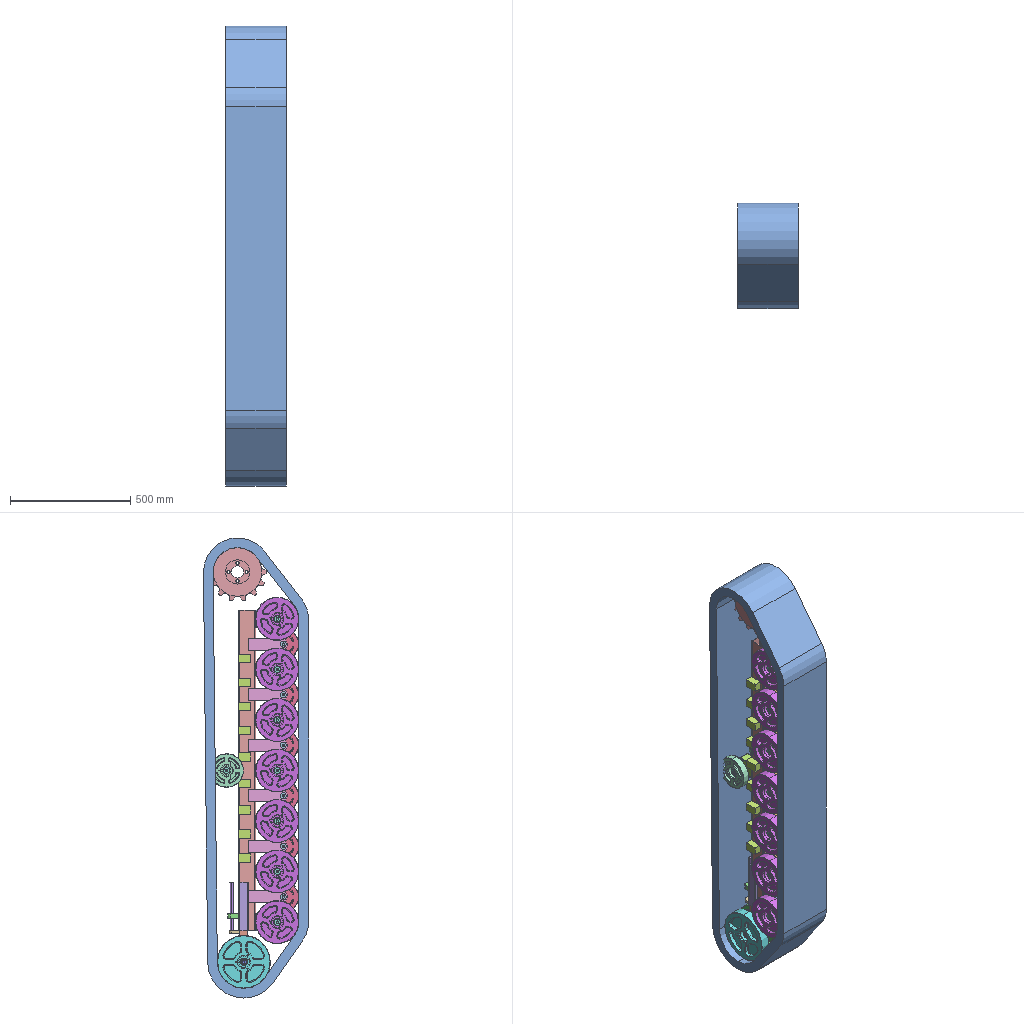Assembly | SolidWorks | 26 different items | 111 placed | box 250 x 436 x 1911 mm
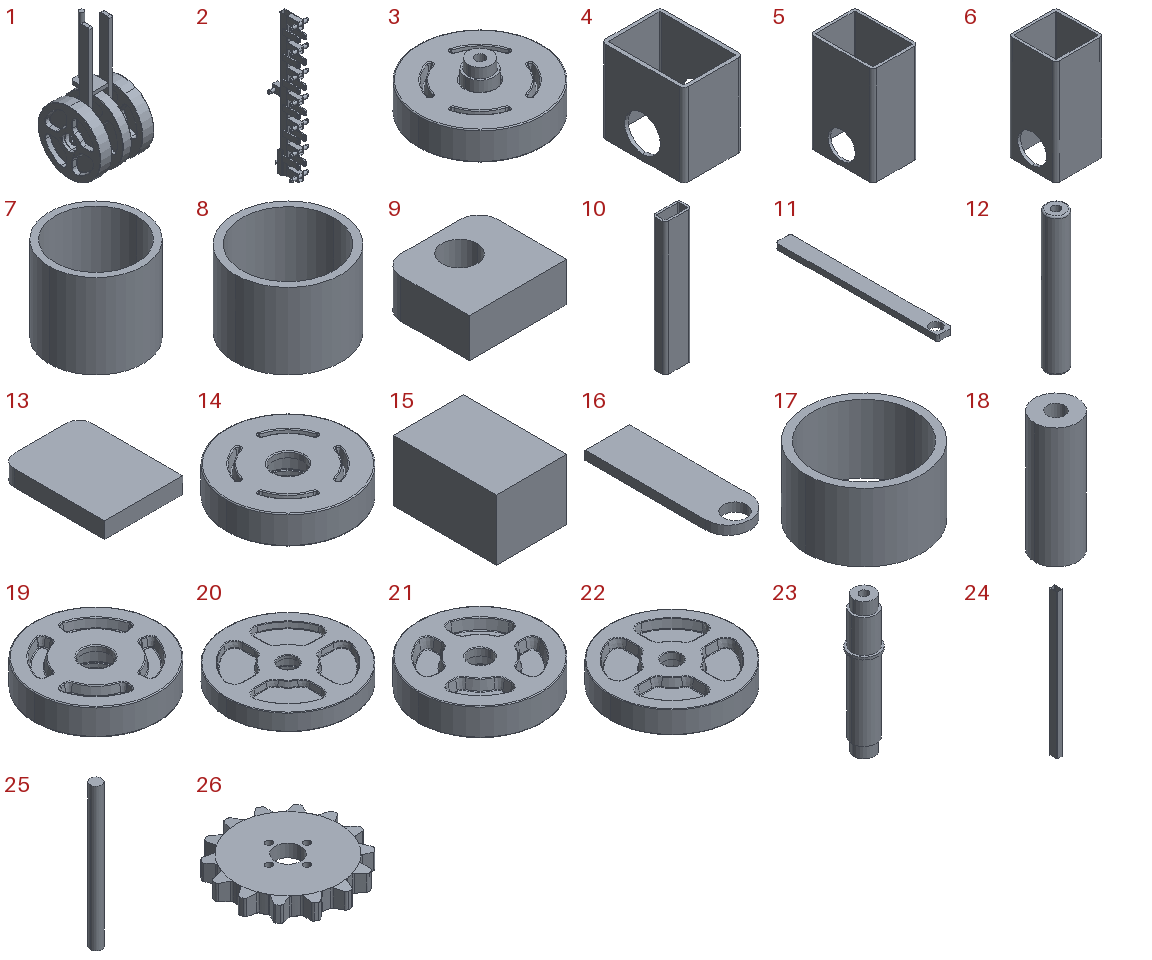Parts list (item | name | quantity | parent item | size | volume | features):
1 | (subassembly) | x1 | - | 188 x 220 x 440 mm | 3274270 mm3 | features CompositeCurve 4
2 | (subassembly) | x1 | - | 166 x 272 x 1330 mm | 3242340 mm3 | features ReferencePattern 20, LocalLPattern 3
3 | (subassembly) | x6 | - | 130 x 130 x 70 mm | 366307 mm3 | -
4 | - | x1 | in 2 | 50 x 70 x 70 mm | 42681 mm3 | features ExtruThin 1, ICE 1
5 | - | x2 | in 2 | 50 x 70 x 110 mm | 69526 mm3 | features ExtruThin 1, ICE 1
6 | - | x5 | in 2 | 50 x 50 x 110 mm | 56326 mm3 | features ExtruThin 1, ICE 1
7 | - | x2 | in 1 | 30 x 30 x 27 mm | 4750 mm3 | features Extrusion 1
8 | - | x2 | in 1 | 30 x 30 x 21.5 mm | 3782 mm3 | features Extrusion 1
9 | - | x1 | in 2 | 50 x 45 x 20 mm | 39052 mm3 | features Extrusion 1, Fillet 1
10 | - | x2 | in 2 | 40 x 20 x 200 mm | 61195 mm3 | features Extrusion 1
11 | - | x2 | in 1 | 32 x 350 x 12 mm | 128014 mm3 | features Extrusion 1
12 | - | x1 | in 1 | 25 x 25 x 166 mm | 76285 mm3 | features HoleWzd 2, Extrusion 1, Fillet 1
13 | - | x1 | in 1 | 58 x 77 x 12 mm | 53077 mm3 | features Extrusion 1, Fillet 1
14 | - | x6 | in 3 | 130 x 130 x 30 mm | 330858 mm3 | features ICE 7, Fillet 2, CirPattern 1, Extrusion 1, MirrorPattern 1
15 | - | x18 | - | 34.866 x 50.94 x 30 mm | 53282 mm3 | features Extrusion 1
16 | - | x12 | in 2 | 50 x 162 x 10 mm | 73008 mm3 | features Extrusion 1, ICE 1
17 | - | x12 | in 3 | 30 x 30 x 17.5 mm | 3079 mm3 | features Extrusion 1
18 | - | x6 | in 3 | 25 x 25 x 70 mm | 29291 mm3 | features HoleWzd 2, Extrusion 1
19 | - | x2 | - | 140 x 140 x 30 mm | 347987 mm3 | features ICE 7, Fillet 2, CirPattern 1, Extrusion 1, MirrorPattern 1
20 | - | x1 | in 1 | 220 x 220 x 30 mm | 789072 mm3 | features ICE 7, Fillet 2, CirPattern 1, Extrusion 1, MirrorPattern 1
21 | - | x14 | - | 180 x 180 x 40 mm | 747348 mm3 | features ICE 7, Fillet 2, CirPattern 1, Extrusion 1, MirrorPattern 1
22 | - | x2 | in 1 | 220 x 220 x 40 mm | 1021265 mm3 | features ICE 7, Fillet 2, CirPattern 1, Extrusion 1, MirrorPattern 1
23 | - | x8 | in 2 | 35 x 35 x 166 mm | 106106 mm3 | features HoleWzd 2, ICE 2, Extrusion 1, MirrorPattern 1
24 | - | x1 | in 2 | 50 x 70 x 1330 mm | 892595 mm3 | features ExtruThin 1
25 | - | x1 | in 1 | 16 x 16 x 200 mm | 40212 mm3 | features Extrusion 1
26 | - | x1 | - | 238.389 x 243 x 35 mm | 1174087 mm3 | features ICE 4, CirPattern 1, Extrusion 1, RevCut 1
Mates (type | each side: item.copy, entity, surface, feature):
In the top assembly
Concentric | 16.1 face cylinder Cut-Extrude1 | 18.1 face cylinder Boss-Extrude1
Coincident | 16.1 face plane Boss-Extrude1 | 17.1 face plane Boss-Extrude1
Concentric | 21.1 face cylinder Boss-Extrude1 | 21.2 face cylinder Boss-Extrude1
Concentric | assembly face | 21.1 face cylinder Boss-Extrude1
Coincident | assembly face | 21.1 face plane Cut-Extrude3
Coincident | assembly face | 21.2 face plane Cut-Extrude3
Concentric | 19.1 face cylinder Boss-Extrude1 | 19.2 face cylinder Boss-Extrude1
Concentric | 23.1 face cylinder Boss-Extrude1 | 19.2 face cylinder Boss-Extrude1
Coincident | 23.1 face plane Boss-Extrude1 | 19.2 face plane Cut-Extrude3
Coincident | 23.1 face plane Boss-Extrude1 | 19.1 face plane Cut-Extrude3
Concentric | 9.1 face cylinder Boss-Extrude1 | 25.1 face cylinder Boss-Extrude1
Parallel | 10.1 face plane Boss-Extrude1 | 11.1 face plane Boss-Extrude1
Coincident | 24.1 face plane Extrude-Thin1 | 13.1 face plane Boss-Extrude1
DistanceDim | 26.1 face plane Boss-Extrude1 | 24.1 face plane Extrude-Thin1
Concentric | 23.2 face cylinder Boss-Extrude2 | 21.2 face cylinder Boss-Extrude1
Coincident | 24.1 face plane Extrude-Thin1 | 15.1 face plane Boss-Extrude1 | 2 times
In subassembly 2
Coincident | 24.2 face plane Extrude-Thin1 | 5.1 face plane Extrude-Thin1 | 3 times
Coincident | 24.2 face plane Extrude-Thin1 | 4.1 face plane Extrude-Thin1 | 2 times
DistanceDim | 4.1 face plane Extrude-Thin1 | 24.2 face plane Extrude-Thin1
Coincident | 16.2 face plane Boss-Extrude1 | 16.3 face plane Boss-Extrude1 | 2 times
Coincident | 24.2 face plane Extrude-Thin1 | 16.3 face plane Boss-Extrude1
Coincident | 24.2 face plane Extrude-Thin1 | 16.2 face plane Boss-Extrude1
DistanceDim | 16.2 face plane Boss-Extrude1 | 24.2 face plane Extrude-Thin1
DistanceDim | 16.2 face plane Boss-Extrude1 | 5.1 face plane Extrude-Thin1
Concentric | 4.1 face cylinder Cut-Extrude1 | 23.3 face cylinder Boss-Extrude1
Coincident | 4.1 face plane Extrude-Thin1 | 23.3 face plane Boss-Extrude4
Coincident | 24.2 face plane Extrude-Thin1 | 5.2 face plane Extrude-Thin1 | 3 times
Coincident | 24.2 face plane Extrude-Thin1 | 6.1 face plane Extrude-Thin1 | 2 times
DistanceDim | 5.1 face plane Extrude-Thin1 | 6.1 face plane Extrude-Thin1
Concentric | 23.4 face cylinder Boss-Extrude1 | 5.2 face cylinder Cut-Extrude1
Coincident | 23.4 face plane Boss-Extrude4 | 5.2 face plane Extrude-Thin1
Coincident | 10.2 face plane Boss-Extrude1 | 10.3 face plane Boss-Extrude1 | 2 times
Coincident | 24.2 face plane Extrude-Thin1 | 10.3 face plane Boss-Extrude1 | 2 times
Coincident | 24.2 face plane Extrude-Thin1 | 10.2 face plane Boss-Extrude1 | 2 times
Coincident | 24.2 face plane Extrude-Thin1 | 9.2 face plane Boss-Extrude1 | 2 times
DistanceDim | 9.2 face plane Boss-Extrude1 | 5.2 face plane Extrude-Thin1
In subassembly 3
Concentric | 14.1 face cylinder Boss-Extrude1 | 18.2 face cylinder Boss-Extrude1
Concentric | 17.2 face cylinder Boss-Extrude1 | 17.3 face cylinder Boss-Extrude1
Concentric | 14.1 face cylinder Boss-Extrude1 | 17.3 face cylinder Boss-Extrude1
In subassembly 1
Coincident | 11.2 face cylinder Boss-Extrude1 | 11.3 edge
Coincident | 11.2 face plane Boss-Extrude1 | 11.3 face plane Boss-Extrude1
Concentric | 7.1 face cylinder Boss-Extrude1 | 7.2 face cylinder Boss-Extrude1
Concentric | 12.1 face cylinder Boss-Extrude1 | 7.2 face cylinder Boss-Extrude1
Concentric | 11.2 face cylinder Boss-Extrude1 | 12.1 face cylinder Boss-Extrude1
Coincident | 11.2 face plane Boss-Extrude1 | 7.2 face plane Boss-Extrude1
Coincident | 11.3 face plane Boss-Extrude1 | 7.1 face plane Boss-Extrude1
Concentric | 8.1 face cylinder Boss-Extrude1 | 8.2 face cylinder Boss-Extrude1
Concentric | 7.2 face cylinder Boss-Extrude1 | 8.2 face cylinder Boss-Extrude1
Coincident | 11.3 face plane Boss-Extrude1 | 8.2 face plane Boss-Extrude1
Coincident | 11.2 face plane Boss-Extrude1 | 8.1 face plane Boss-Extrude1
Coincident | 22.1 face cylinder Boss-Extrude1 | 22.2 edge
Coincident | 7.1 face plane Boss-Extrude1 | 22.2 face plane Cut-Extrude3
Coincident | 7.2 face plane Boss-Extrude1 | 22.1 face plane Cut-Extrude3
Coincident | 12.1 face plane Boss-Extrude1 | 22.1 edge
Coincident | 11.3 face plane Boss-Extrude1 | 13.2 face plane Boss-Extrude1 | 2 times
DistanceDim | 13.2 face plane Boss-Extrude1 | 11.3 face plane Boss-Extrude1
Coincident | 11.2 face plane Boss-Extrude1 | 13.2 face plane Boss-Extrude1
Coincident | 13.2 face plane Boss-Extrude1 | 25.2 face plane Boss-Extrude1
Concentric | 13.2 select_type:25 | 25.2 face cylinder Boss-Extrude1
Concentric | 22.2 face cylinder Boss-Extrude1 | 20.1 face cylinder Boss-Extrude1
Concentric | 8.1 edge | 22.2 face cylinder Boss-Extrude1
Coincident | 8.1 face plane Boss-Extrude1 | 20.1 face plane Cut-Extrude4
Coincident | 13.2 face plane Boss-Extrude1 | 1.1 plane